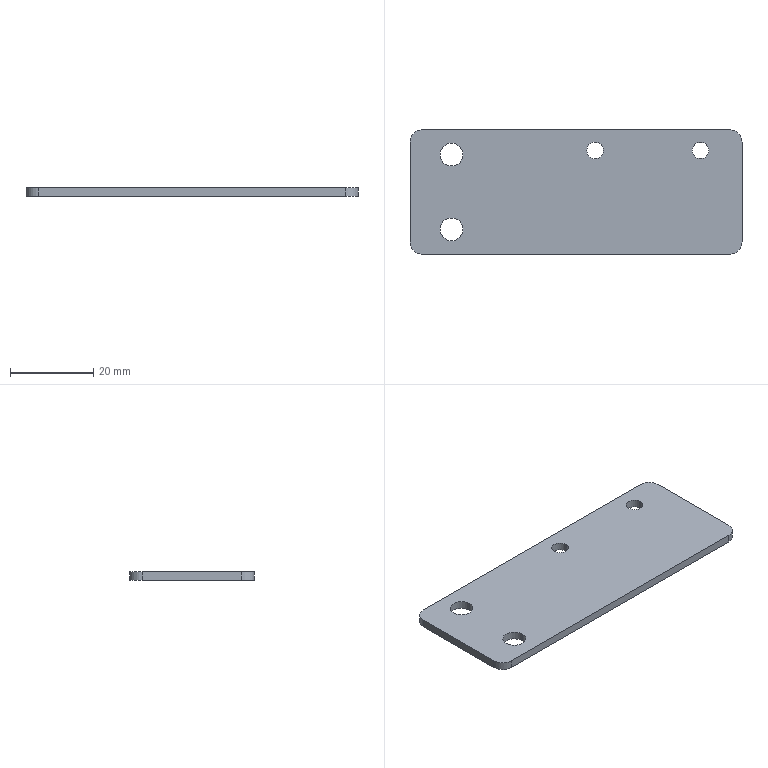Part | SolidWorks | features HoleWzd 2, Fillet 1, FlatPattern 1, SMBaseFlange 1, SheetMetal 1 | 1 solid | 18 faces | box 80 x 30 x 2 mm | volume 4639 mm3 | cylinder 12 | plane 6 | commonest cylinder face diameters 4 x4 5.5 x4 6 x4
STEP:
#1=CARTESIAN_POINT('',(7.25,24.,-2.));
#2=VERTEX_POINT('',#1);
#3=CARTESIAN_POINT('',(12.75,24.,-2.));
#4=VERTEX_POINT('',#3);
#5=CARTESIAN_POINT('',(10.,24.,-2.));
#6=DIRECTION('',(0.,0.,1.));
#7=DIRECTION('',(1.,0.,0.));
#8=AXIS2_PLACEMENT_3D('',#5,#6,#7);
#9=CIRCLE('',#8,2.75);
#10=EDGE_CURVE('',#2,#4,#9,.T.);
#11=ORIENTED_EDGE('',*,*,#10,.F.);
#12=CARTESIAN_POINT('',(7.25,24.,0.));
#13=VERTEX_POINT('',#12);
#14=CARTESIAN_POINT('',(7.25,24.,0.));
#15=DIRECTION('',(0.,0.,1.));
#16=VECTOR('',#15,1000.);
#17=LINE('',#14,#16);
#18=EDGE_CURVE('',#2,#13,#17,.T.);
#19=ORIENTED_EDGE('',*,*,#18,.T.);
#20=CARTESIAN_POINT('',(12.75,24.,0.));
#21=VERTEX_POINT('',#20);
#22=CARTESIAN_POINT('',(10.,24.,0.));
#23=DIRECTION('',(0.,0.,1.));
#24=DIRECTION('',(1.,0.,0.));
#25=AXIS2_PLACEMENT_3D('',#22,#23,#24);
#26=CIRCLE('',#25,2.75);
#27=EDGE_CURVE('',#13,#21,#26,.T.);
#28=ORIENTED_EDGE('',*,*,#27,.T.);
#29=CARTESIAN_POINT('',(12.75,24.,0.));
#30=DIRECTION('',(0.,0.,1.));
#31=VECTOR('',#30,1000.);
#32=LINE('',#29,#31);
#33=EDGE_CURVE('',#4,#21,#32,.T.);
#34=ORIENTED_EDGE('',*,*,#33,.F.);
#35=EDGE_LOOP('',(#11,#19,#28,#34));
#36=FACE_OUTER_BOUND('',#35,.T.);
#37=CARTESIAN_POINT('',(10.,24.,0.));
#38=DIRECTION('',(0.,0.,1.));
#39=DIRECTION('',(1.,0.,0.));
#40=AXIS2_PLACEMENT_3D('',#37,#38,#39);
#41=CYLINDRICAL_SURFACE('',#40,2.75);
#42=ADVANCED_FACE('',(#36),#41,.F.);
#43=CARTESIAN_POINT('',(7.25,6.,-2.));
#44=VERTEX_POINT('',#43);
#45=CARTESIAN_POINT('',(12.75,6.,-2.));
#46=VERTEX_POINT('',#45);
#47=CARTESIAN_POINT('',(10.,6.,-2.));
#48=DIRECTION('',(0.,0.,1.));
#49=DIRECTION('',(1.,0.,0.));
#50=AXIS2_PLACEMENT_3D('',#47,#48,#49);
#51=CIRCLE('',#50,2.75);
#52=EDGE_CURVE('',#44,#46,#51,.T.);
#53=ORIENTED_EDGE('',*,*,#52,.F.);
#54=CARTESIAN_POINT('',(7.25,6.,0.));
#55=VERTEX_POINT('',#54);
#56=CARTESIAN_POINT('',(7.25,6.,0.));
#57=DIRECTION('',(0.,0.,1.));
#58=VECTOR('',#57,1000.);
#59=LINE('',#56,#58);
#60=EDGE_CURVE('',#44,#55,#59,.T.);
#61=ORIENTED_EDGE('',*,*,#60,.T.);
#62=CARTESIAN_POINT('',(12.75,6.,0.));
#63=VERTEX_POINT('',#62);
#64=CARTESIAN_POINT('',(10.,6.,0.));
#65=DIRECTION('',(0.,0.,1.));
#66=DIRECTION('',(1.,0.,0.));
#67=AXIS2_PLACEMENT_3D('',#64,#65,#66);
#68=CIRCLE('',#67,2.75);
#69=EDGE_CURVE('',#55,#63,#68,.T.);
#70=ORIENTED_EDGE('',*,*,#69,.T.);
#71=CARTESIAN_POINT('',(12.75,6.,0.));
#72=DIRECTION('',(0.,0.,1.));
#73=VECTOR('',#72,1000.);
#74=LINE('',#71,#73);
#75=EDGE_CURVE('',#46,#63,#74,.T.);
#76=ORIENTED_EDGE('',*,*,#75,.F.);
#77=EDGE_LOOP('',(#53,#61,#70,#76));
#78=FACE_OUTER_BOUND('',#77,.T.);
#79=CARTESIAN_POINT('',(10.,6.,0.));
#80=DIRECTION('',(0.,0.,1.));
#81=DIRECTION('',(1.,0.,0.));
#82=AXIS2_PLACEMENT_3D('',#79,#80,#81);
#83=CYLINDRICAL_SURFACE('',#82,2.75);
#84=ADVANCED_FACE('',(#78),#83,.F.);
#85=CARTESIAN_POINT('',(72.,25.,-2.));
#86=VERTEX_POINT('',#85);
#87=CARTESIAN_POINT('',(68.,25.,-2.));
#88=VERTEX_POINT('',#87);
#89=CARTESIAN_POINT('',(70.,25.,-2.));
#90=DIRECTION('',(0.,0.,-1.));
#91=DIRECTION('',(-1.,0.,0.));
#92=AXIS2_PLACEMENT_3D('',#89,#90,#91);
#93=CIRCLE('',#92,2.);
#94=EDGE_CURVE('',#86,#88,#93,.T.);
#95=ORIENTED_EDGE('',*,*,#94,.T.);
#96=CARTESIAN_POINT('',(68.,25.,0.));
#97=VERTEX_POINT('',#96);
#98=CARTESIAN_POINT('',(68.,25.,0.));
#99=DIRECTION('',(0.,0.,1.));
#100=VECTOR('',#99,1000.);
#101=LINE('',#98,#100);
#102=EDGE_CURVE('',#88,#97,#101,.T.);
#103=ORIENTED_EDGE('',*,*,#102,.T.);
#104=CARTESIAN_POINT('',(72.,25.,0.));
#105=VERTEX_POINT('',#104);
#106=CARTESIAN_POINT('',(70.,25.,0.));
#107=DIRECTION('',(0.,0.,1.));
#108=DIRECTION('',(1.,0.,0.));
#109=AXIS2_PLACEMENT_3D('',#106,#107,#108);
#110=CIRCLE('',#109,2.);
#111=EDGE_CURVE('',#97,#105,#110,.T.);
#112=ORIENTED_EDGE('',*,*,#111,.T.);
#113=CARTESIAN_POINT('',(72.,25.,0.));
#114=DIRECTION('',(0.,0.,1.));
#115=VECTOR('',#114,1000.);
#116=LINE('',#113,#115);
#117=EDGE_CURVE('',#86,#105,#116,.T.);
#118=ORIENTED_EDGE('',*,*,#117,.F.);
#119=EDGE_LOOP('',(#95,#103,#112,#118));
#120=FACE_OUTER_BOUND('',#119,.T.);
#121=CARTESIAN_POINT('',(70.,25.,0.));
#122=DIRECTION('',(0.,0.,1.));
#123=DIRECTION('',(1.,0.,0.));
#124=AXIS2_PLACEMENT_3D('',#121,#122,#123);
#125=CYLINDRICAL_SURFACE('',#124,2.);
#126=ADVANCED_FACE('',(#120),#125,.F.);
#127=CARTESIAN_POINT('',(46.6,25.,-2.));
#128=VERTEX_POINT('',#127);
#129=CARTESIAN_POINT('',(42.6,25.,-2.));
#130=VERTEX_POINT('',#129);
#131=CARTESIAN_POINT('',(44.6,25.,-2.));
#132=DIRECTION('',(0.,0.,-1.));
#133=DIRECTION('',(-1.,0.,0.));
#134=AXIS2_PLACEMENT_3D('',#131,#132,#133);
#135=CIRCLE('',#134,2.);
#136=EDGE_CURVE('',#128,#130,#135,.T.);
#137=ORIENTED_EDGE('',*,*,#136,.T.);
#138=CARTESIAN_POINT('',(42.6,25.,0.));
#139=VERTEX_POINT('',#138);
#140=CARTESIAN_POINT('',(42.6,25.,0.));
#141=DIRECTION('',(0.,0.,1.));
#142=VECTOR('',#141,1000.);
#143=LINE('',#140,#142);
#144=EDGE_CURVE('',#130,#139,#143,.T.);
#145=ORIENTED_EDGE('',*,*,#144,.T.);
#146=CARTESIAN_POINT('',(46.6,25.,0.));
#147=VERTEX_POINT('',#146);
#148=CARTESIAN_POINT('',(44.6,25.,0.));
#149=DIRECTION('',(0.,0.,1.));
#150=DIRECTION('',(1.,0.,0.));
#151=AXIS2_PLACEMENT_3D('',#148,#149,#150);
#152=CIRCLE('',#151,2.);
#153=EDGE_CURVE('',#139,#147,#152,.T.);
#154=ORIENTED_EDGE('',*,*,#153,.T.);
#155=CARTESIAN_POINT('',(46.6,25.,0.));
#156=DIRECTION('',(0.,0.,1.));
#157=VECTOR('',#156,1000.);
#158=LINE('',#155,#157);
#159=EDGE_CURVE('',#128,#147,#158,.T.);
#160=ORIENTED_EDGE('',*,*,#159,.F.);
#161=EDGE_LOOP('',(#137,#145,#154,#160));
#162=FACE_OUTER_BOUND('',#161,.T.);
#163=CARTESIAN_POINT('',(44.6,25.,0.));
#164=DIRECTION('',(0.,0.,1.));
#165=DIRECTION('',(1.,0.,0.));
#166=AXIS2_PLACEMENT_3D('',#163,#164,#165);
#167=CYLINDRICAL_SURFACE('',#166,2.);
#168=ADVANCED_FACE('',(#162),#167,.F.);
#169=CARTESIAN_POINT('',(0.,27.,-2.));
#170=VERTEX_POINT('',#169);
#171=CARTESIAN_POINT('',(0.,3.,-2.));
#172=VERTEX_POINT('',#171);
#173=CARTESIAN_POINT('',(0.,0.,-2.));
#174=DIRECTION('',(0.,-1.,0.));
#175=VECTOR('',#174,1000.);
#176=LINE('',#173,#175);
#177=EDGE_CURVE('',#170,#172,#176,.T.);
#178=ORIENTED_EDGE('',*,*,#177,.T.);
#179=CARTESIAN_POINT('',(0.,3.,0.));
#180=VERTEX_POINT('',#179);
#181=CARTESIAN_POINT('',(0.,3.,-2.));
#182=DIRECTION('',(0.,0.,1.));
#183=VECTOR('',#182,1000.);
#184=LINE('',#181,#183);
#185=EDGE_CURVE('',#172,#180,#184,.T.);
#186=ORIENTED_EDGE('',*,*,#185,.T.);
#187=CARTESIAN_POINT('',(0.,27.,0.));
#188=VERTEX_POINT('',#187);
#189=CARTESIAN_POINT('',(0.,0.,0.));
#190=DIRECTION('',(0.,-1.,0.));
#191=VECTOR('',#190,1000.);
#192=LINE('',#189,#191);
#193=EDGE_CURVE('',#188,#180,#192,.T.);
#194=ORIENTED_EDGE('',*,*,#193,.F.);
#195=CARTESIAN_POINT('',(0.,27.,-2.));
#196=DIRECTION('',(0.,0.,-1.));
#197=VECTOR('',#196,1000.);
#198=LINE('',#195,#197);
#199=EDGE_CURVE('',#188,#170,#198,.T.);
#200=ORIENTED_EDGE('',*,*,#199,.T.);
#201=EDGE_LOOP('',(#178,#186,#194,#200));
#202=FACE_OUTER_BOUND('',#201,.T.);
#203=CARTESIAN_POINT('',(0.,0.,-2.));
#204=DIRECTION('',(-1.,0.,0.));
#205=DIRECTION('',(0.,0.,1.));
#206=AXIS2_PLACEMENT_3D('',#203,#204,#205);
#207=PLANE('',#206);
#208=ADVANCED_FACE('',(#202),#207,.T.);
#209=CARTESIAN_POINT('',(77.,30.,0.));
#210=VERTEX_POINT('',#209);
#211=CARTESIAN_POINT('',(3.,30.,0.));
#212=VERTEX_POINT('',#211);
#213=CARTESIAN_POINT('',(0.,30.,0.));
#214=DIRECTION('',(-1.,0.,0.));
#215=VECTOR('',#214,1000.);
#216=LINE('',#213,#215);
#217=EDGE_CURVE('',#210,#212,#216,.T.);
#218=ORIENTED_EDGE('',*,*,#217,.F.);
#219=CARTESIAN_POINT('',(77.,30.,-2.));
#220=VERTEX_POINT('',#219);
#221=CARTESIAN_POINT('',(77.,30.,-2.));
#222=DIRECTION('',(0.,0.,-1.));
#223=VECTOR('',#222,1000.);
#224=LINE('',#221,#223);
#225=EDGE_CURVE('',#210,#220,#224,.T.);
#226=ORIENTED_EDGE('',*,*,#225,.T.);
#227=CARTESIAN_POINT('',(3.,30.,-2.));
#228=VERTEX_POINT('',#227);
#229=CARTESIAN_POINT('',(0.,30.,-2.));
#230=DIRECTION('',(-1.,0.,0.));
#231=VECTOR('',#230,1000.);
#232=LINE('',#229,#231);
#233=EDGE_CURVE('',#220,#228,#232,.T.);
#234=ORIENTED_EDGE('',*,*,#233,.T.);
#235=CARTESIAN_POINT('',(3.,30.,-2.));
#236=DIRECTION('',(0.,0.,1.));
#237=VECTOR('',#236,1000.);
#238=LINE('',#235,#237);
#239=EDGE_CURVE('',#228,#212,#238,.T.);
#240=ORIENTED_EDGE('',*,*,#239,.T.);
#241=EDGE_LOOP('',(#218,#226,#234,#240));
#242=FACE_OUTER_BOUND('',#241,.T.);
#243=CARTESIAN_POINT('',(0.,30.,-2.));
#244=DIRECTION('',(0.,1.,0.));
#245=DIRECTION('',(0.,0.,1.));
#246=AXIS2_PLACEMENT_3D('',#243,#244,#245);
#247=PLANE('',#246);
#248=ADVANCED_FACE('',(#242),#247,.T.);
#249=CARTESIAN_POINT('',(80.,3.,0.));
#250=VERTEX_POINT('',#249);
#251=CARTESIAN_POINT('',(80.,27.,0.));
#252=VERTEX_POINT('',#251);
#253=CARTESIAN_POINT('',(80.,0.,0.));
#254=DIRECTION('',(0.,1.,0.));
#255=VECTOR('',#254,1000.);
#256=LINE('',#253,#255);
#257=EDGE_CURVE('',#250,#252,#256,.T.);
#258=ORIENTED_EDGE('',*,*,#257,.F.);
#259=CARTESIAN_POINT('',(80.,3.,-2.));
#260=VERTEX_POINT('',#259);
#261=CARTESIAN_POINT('',(80.,3.,-2.));
#262=DIRECTION('',(0.,0.,-1.));
#263=VECTOR('',#262,1000.);
#264=LINE('',#261,#263);
#265=EDGE_CURVE('',#250,#260,#264,.T.);
#266=ORIENTED_EDGE('',*,*,#265,.T.);
#267=CARTESIAN_POINT('',(80.,27.,-2.));
#268=VERTEX_POINT('',#267);
#269=CARTESIAN_POINT('',(80.,0.,-2.));
#270=DIRECTION('',(0.,1.,0.));
#271=VECTOR('',#270,1000.);
#272=LINE('',#269,#271);
#273=EDGE_CURVE('',#260,#268,#272,.T.);
#274=ORIENTED_EDGE('',*,*,#273,.T.);
#275=CARTESIAN_POINT('',(80.,27.,-2.));
#276=DIRECTION('',(0.,0.,1.));
#277=VECTOR('',#276,1000.);
#278=LINE('',#275,#277);
#279=EDGE_CURVE('',#268,#252,#278,.T.);
#280=ORIENTED_EDGE('',*,*,#279,.T.);
#281=EDGE_LOOP('',(#258,#266,#274,#280));
#282=FACE_OUTER_BOUND('',#281,.T.);
#283=CARTESIAN_POINT('',(80.,0.,-2.));
#284=DIRECTION('',(1.,0.,0.));
#285=DIRECTION('',(0.,0.,-1.));
#286=AXIS2_PLACEMENT_3D('',#283,#284,#285);
#287=PLANE('',#286);
#288=ADVANCED_FACE('',(#282),#287,.T.);
#289=CARTESIAN_POINT('',(3.,0.,-2.));
#290=VERTEX_POINT('',#289);
#291=CARTESIAN_POINT('',(77.,0.,-2.));
#292=VERTEX_POINT('',#291);
#293=CARTESIAN_POINT('',(0.,0.,-2.));
#294=DIRECTION('',(1.,0.,0.));
#295=VECTOR('',#294,1000.);
#296=LINE('',#293,#295);
#297=EDGE_CURVE('',#290,#292,#296,.T.);
#298=ORIENTED_EDGE('',*,*,#297,.T.);
#299=CARTESIAN_POINT('',(77.,0.,0.));
#300=VERTEX_POINT('',#299);
#301=CARTESIAN_POINT('',(77.,0.,-2.));
#302=DIRECTION('',(0.,0.,1.));
#303=VECTOR('',#302,1000.);
#304=LINE('',#301,#303);
#305=EDGE_CURVE('',#292,#300,#304,.T.);
#306=ORIENTED_EDGE('',*,*,#305,.T.);
#307=CARTESIAN_POINT('',(3.,0.,0.));
#308=VERTEX_POINT('',#307);
#309=CARTESIAN_POINT('',(0.,0.,0.));
#310=DIRECTION('',(1.,0.,0.));
#311=VECTOR('',#310,1000.);
#312=LINE('',#309,#311);
#313=EDGE_CURVE('',#308,#300,#312,.T.);
#314=ORIENTED_EDGE('',*,*,#313,.F.);
#315=CARTESIAN_POINT('',(3.,0.,-2.));
#316=DIRECTION('',(0.,0.,-1.));
#317=VECTOR('',#316,1000.);
#318=LINE('',#315,#317);
#319=EDGE_CURVE('',#308,#290,#318,.T.);
#320=ORIENTED_EDGE('',*,*,#319,.T.);
#321=EDGE_LOOP('',(#298,#306,#314,#320));
#322=FACE_OUTER_BOUND('',#321,.T.);
#323=CARTESIAN_POINT('',(0.,0.,-2.));
#324=DIRECTION('',(0.,-1.,0.));
#325=DIRECTION('',(0.,0.,-1.));
#326=AXIS2_PLACEMENT_3D('',#323,#324,#325);
#327=PLANE('',#326);
#328=ADVANCED_FACE('',(#322),#327,.T.);
#329=CARTESIAN_POINT('',(10.,24.,-2.));
#330=DIRECTION('',(0.,0.,1.));
#331=DIRECTION('',(1.,0.,0.));
#332=AXIS2_PLACEMENT_3D('',#329,#330,#331);
#333=CIRCLE('',#332,2.75);
#334=EDGE_CURVE('',#4,#2,#333,.T.);
#335=ORIENTED_EDGE('',*,*,#334,.T.);
#336=ORIENTED_EDGE('',*,*,#10,.T.);
#337=EDGE_LOOP('',(#335,#336));
#338=FACE_BOUND('',#337,.T.);
#339=CARTESIAN_POINT('',(10.,6.,-2.));
#340=DIRECTION('',(0.,0.,1.));
#341=DIRECTION('',(1.,0.,0.));
#342=AXIS2_PLACEMENT_3D('',#339,#340,#341);
#343=CIRCLE('',#342,2.75);
#344=EDGE_CURVE('',#46,#44,#343,.T.);
#345=ORIENTED_EDGE('',*,*,#344,.T.);
#346=ORIENTED_EDGE('',*,*,#52,.T.);
#347=EDGE_LOOP('',(#345,#346));
#348=FACE_BOUND('',#347,.T.);
#349=ORIENTED_EDGE('',*,*,#94,.F.);
#350=CARTESIAN_POINT('',(70.,25.,-2.));
#351=DIRECTION('',(0.,0.,-1.));
#352=DIRECTION('',(-1.,0.,0.));
#353=AXIS2_PLACEMENT_3D('',#350,#351,#352);
#354=CIRCLE('',#353,2.);
#355=EDGE_CURVE('',#88,#86,#354,.T.);
#356=ORIENTED_EDGE('',*,*,#355,.F.);
#357=EDGE_LOOP('',(#349,#356));
#358=FACE_BOUND('',#357,.T.);
#359=ORIENTED_EDGE('',*,*,#136,.F.);
#360=CARTESIAN_POINT('',(44.6,25.,-2.));
#361=DIRECTION('',(0.,0.,-1.));
#362=DIRECTION('',(-1.,0.,0.));
#363=AXIS2_PLACEMENT_3D('',#360,#361,#362);
#364=CIRCLE('',#363,2.);
#365=EDGE_CURVE('',#130,#128,#364,.T.);
#366=ORIENTED_EDGE('',*,*,#365,.F.);
#367=EDGE_LOOP('',(#359,#366));
#368=FACE_BOUND('',#367,.T.);
#369=ORIENTED_EDGE('',*,*,#273,.F.);
#370=CARTESIAN_POINT('',(77.,3.,-2.));
#371=DIRECTION('',(0.,0.,-1.));
#372=DIRECTION('',(-1.,0.,0.));
#373=AXIS2_PLACEMENT_3D('',#370,#371,#372);
#374=CIRCLE('',#373,3.);
#375=EDGE_CURVE('',#260,#292,#374,.T.);
#376=ORIENTED_EDGE('',*,*,#375,.T.);
#377=ORIENTED_EDGE('',*,*,#297,.F.);
#378=CARTESIAN_POINT('',(3.,3.,-2.));
#379=DIRECTION('',(0.,0.,-1.));
#380=DIRECTION('',(-1.,0.,0.));
#381=AXIS2_PLACEMENT_3D('',#378,#379,#380);
#382=CIRCLE('',#381,3.);
#383=EDGE_CURVE('',#290,#172,#382,.T.);
#384=ORIENTED_EDGE('',*,*,#383,.T.);
#385=ORIENTED_EDGE('',*,*,#177,.F.);
#386=CARTESIAN_POINT('',(3.,27.,-2.));
#387=DIRECTION('',(0.,0.,-1.));
#388=DIRECTION('',(-1.,0.,0.));
#389=AXIS2_PLACEMENT_3D('',#386,#387,#388);
#390=CIRCLE('',#389,3.);
#391=EDGE_CURVE('',#170,#228,#390,.T.);
#392=ORIENTED_EDGE('',*,*,#391,.T.);
#393=ORIENTED_EDGE('',*,*,#233,.F.);
#394=CARTESIAN_POINT('',(77.,27.,-2.));
#395=DIRECTION('',(0.,0.,-1.));
#396=DIRECTION('',(-1.,0.,0.));
#397=AXIS2_PLACEMENT_3D('',#394,#395,#396);
#398=CIRCLE('',#397,3.);
#399=EDGE_CURVE('',#220,#268,#398,.T.);
#400=ORIENTED_EDGE('',*,*,#399,.T.);
#401=EDGE_LOOP('',(#369,#376,#377,#384,#385,#392,#393,#400));
#402=FACE_OUTER_BOUND('',#401,.T.);
#403=CARTESIAN_POINT('',(0.,0.,-2.));
#404=DIRECTION('',(0.,0.,-1.));
#405=DIRECTION('',(-1.,0.,0.));
#406=AXIS2_PLACEMENT_3D('',#403,#404,#405);
#407=PLANE('',#406);
#408=ADVANCED_FACE('',(#338,#348,#358,#368,#402),#407,.T.);
#409=CARTESIAN_POINT('',(10.,24.,0.));
#410=DIRECTION('',(0.,0.,1.));
#411=DIRECTION('',(1.,0.,0.));
#412=AXIS2_PLACEMENT_3D('',#409,#410,#411);
#413=CIRCLE('',#412,2.75);
#414=EDGE_CURVE('',#21,#13,#413,.T.);
#415=ORIENTED_EDGE('',*,*,#414,.F.);
#416=ORIENTED_EDGE('',*,*,#27,.F.);
#417=EDGE_LOOP('',(#415,#416));
#418=FACE_BOUND('',#417,.T.);
#419=CARTESIAN_POINT('',(10.,6.,0.));
#420=DIRECTION('',(0.,0.,1.));
#421=DIRECTION('',(1.,0.,0.));
#422=AXIS2_PLACEMENT_3D('',#419,#420,#421);
#423=CIRCLE('',#422,2.75);
#424=EDGE_CURVE('',#63,#55,#423,.T.);
#425=ORIENTED_EDGE('',*,*,#424,.F.);
#426=ORIENTED_EDGE('',*,*,#69,.F.);
#427=EDGE_LOOP('',(#425,#426));
#428=FACE_BOUND('',#427,.T.);
#429=CARTESIAN_POINT('',(70.,25.,0.));
#430=DIRECTION('',(0.,0.,1.));
#431=DIRECTION('',(1.,0.,0.));
#432=AXIS2_PLACEMENT_3D('',#429,#430,#431);
#433=CIRCLE('',#432,2.);
#434=EDGE_CURVE('',#105,#97,#433,.T.);
#435=ORIENTED_EDGE('',*,*,#434,.F.);
#436=ORIENTED_EDGE('',*,*,#111,.F.);
#437=EDGE_LOOP('',(#435,#436));
#438=FACE_BOUND('',#437,.T.);
#439=CARTESIAN_POINT('',(44.6,25.,0.));
#440=DIRECTION('',(0.,0.,1.));
#441=DIRECTION('',(1.,0.,0.));
#442=AXIS2_PLACEMENT_3D('',#439,#440,#441);
#443=CIRCLE('',#442,2.);
#444=EDGE_CURVE('',#147,#139,#443,.T.);
#445=ORIENTED_EDGE('',*,*,#444,.F.);
#446=ORIENTED_EDGE('',*,*,#153,.F.);
#447=EDGE_LOOP('',(#445,#446));
#448=FACE_BOUND('',#447,.T.);
#449=ORIENTED_EDGE('',*,*,#313,.T.);
#450=CARTESIAN_POINT('',(77.,3.,0.));
#451=DIRECTION('',(0.,0.,1.));
#452=DIRECTION('',(-1.,0.,0.));
#453=AXIS2_PLACEMENT_3D('',#450,#451,#452);
#454=CIRCLE('',#453,3.);
#455=EDGE_CURVE('',#300,#250,#454,.T.);
#456=ORIENTED_EDGE('',*,*,#455,.T.);
#457=ORIENTED_EDGE('',*,*,#257,.T.);
#458=CARTESIAN_POINT('',(77.,27.,0.));
#459=DIRECTION('',(0.,0.,1.));
#460=DIRECTION('',(-1.,0.,0.));
#461=AXIS2_PLACEMENT_3D('',#458,#459,#460);
#462=CIRCLE('',#461,3.);
#463=EDGE_CURVE('',#252,#210,#462,.T.);
#464=ORIENTED_EDGE('',*,*,#463,.T.);
#465=ORIENTED_EDGE('',*,*,#217,.T.);
#466=CARTESIAN_POINT('',(3.,27.,0.));
#467=DIRECTION('',(0.,0.,1.));
#468=DIRECTION('',(-1.,0.,0.));
#469=AXIS2_PLACEMENT_3D('',#466,#467,#468);
#470=CIRCLE('',#469,3.);
#471=EDGE_CURVE('',#212,#188,#470,.T.);
#472=ORIENTED_EDGE('',*,*,#471,.T.);
#473=ORIENTED_EDGE('',*,*,#193,.T.);
#474=CARTESIAN_POINT('',(3.,3.,0.));
#475=DIRECTION('',(0.,0.,1.));
#476=DIRECTION('',(-1.,0.,0.));
#477=AXIS2_PLACEMENT_3D('',#474,#475,#476);
#478=CIRCLE('',#477,3.);
#479=EDGE_CURVE('',#180,#308,#478,.T.);
#480=ORIENTED_EDGE('',*,*,#479,.T.);
#481=EDGE_LOOP('',(#449,#456,#457,#464,#465,#472,#473,#480));
#482=FACE_OUTER_BOUND('',#481,.T.);
#483=CARTESIAN_POINT('',(0.,0.,0.));
#484=DIRECTION('',(0.,0.,-1.));
#485=DIRECTION('',(-1.,0.,0.));
#486=AXIS2_PLACEMENT_3D('',#483,#484,#485);
#487=PLANE('',#486);
#488=ADVANCED_FACE('',(#418,#428,#438,#448,#482),#487,.F.);
#489=ORIENTED_EDGE('',*,*,#144,.F.);
#490=ORIENTED_EDGE('',*,*,#365,.T.);
#491=ORIENTED_EDGE('',*,*,#159,.T.);
#492=ORIENTED_EDGE('',*,*,#444,.T.);
#493=EDGE_LOOP('',(#489,#490,#491,#492));
#494=FACE_OUTER_BOUND('',#493,.T.);
#495=CARTESIAN_POINT('',(44.6,25.,0.));
#496=DIRECTION('',(0.,0.,1.));
#497=DIRECTION('',(1.,0.,0.));
#498=AXIS2_PLACEMENT_3D('',#495,#496,#497);
#499=CYLINDRICAL_SURFACE('',#498,2.);
#500=ADVANCED_FACE('',(#494),#499,.F.);
#501=ORIENTED_EDGE('',*,*,#102,.F.);
#502=ORIENTED_EDGE('',*,*,#355,.T.);
#503=ORIENTED_EDGE('',*,*,#117,.T.);
#504=ORIENTED_EDGE('',*,*,#434,.T.);
#505=EDGE_LOOP('',(#501,#502,#503,#504));
#506=FACE_OUTER_BOUND('',#505,.T.);
#507=CARTESIAN_POINT('',(70.,25.,0.));
#508=DIRECTION('',(0.,0.,1.));
#509=DIRECTION('',(1.,0.,0.));
#510=AXIS2_PLACEMENT_3D('',#507,#508,#509);
#511=CYLINDRICAL_SURFACE('',#510,2.);
#512=ADVANCED_FACE('',(#506),#511,.F.);
#513=ORIENTED_EDGE('',*,*,#60,.F.);
#514=ORIENTED_EDGE('',*,*,#344,.F.);
#515=ORIENTED_EDGE('',*,*,#75,.T.);
#516=ORIENTED_EDGE('',*,*,#424,.T.);
#517=EDGE_LOOP('',(#513,#514,#515,#516));
#518=FACE_OUTER_BOUND('',#517,.T.);
#519=CARTESIAN_POINT('',(10.,6.,0.));
#520=DIRECTION('',(0.,0.,1.));
#521=DIRECTION('',(1.,0.,0.));
#522=AXIS2_PLACEMENT_3D('',#519,#520,#521);
#523=CYLINDRICAL_SURFACE('',#522,2.75);
#524=ADVANCED_FACE('',(#518),#523,.F.);
#525=ORIENTED_EDGE('',*,*,#18,.F.);
#526=ORIENTED_EDGE('',*,*,#334,.F.);
#527=ORIENTED_EDGE('',*,*,#33,.T.);
#528=ORIENTED_EDGE('',*,*,#414,.T.);
#529=EDGE_LOOP('',(#525,#526,#527,#528));
#530=FACE_OUTER_BOUND('',#529,.T.);
#531=CARTESIAN_POINT('',(10.,24.,0.));
#532=DIRECTION('',(0.,0.,1.));
#533=DIRECTION('',(1.,0.,0.));
#534=AXIS2_PLACEMENT_3D('',#531,#532,#533);
#535=CYLINDRICAL_SURFACE('',#534,2.75);
#536=ADVANCED_FACE('',(#530),#535,.F.);
#537=ORIENTED_EDGE('',*,*,#375,.F.);
#538=ORIENTED_EDGE('',*,*,#265,.F.);
#539=ORIENTED_EDGE('',*,*,#455,.F.);
#540=ORIENTED_EDGE('',*,*,#305,.F.);
#541=EDGE_LOOP('',(#537,#538,#539,#540));
#542=FACE_OUTER_BOUND('',#541,.T.);
#543=CARTESIAN_POINT('',(77.,3.,-2.));
#544=DIRECTION('',(0.,0.,1.));
#545=DIRECTION('',(1.,0.,0.));
#546=AXIS2_PLACEMENT_3D('',#543,#544,#545);
#547=CYLINDRICAL_SURFACE('',#546,3.);
#548=ADVANCED_FACE('',(#542),#547,.T.);
#549=ORIENTED_EDGE('',*,*,#399,.F.);
#550=ORIENTED_EDGE('',*,*,#225,.F.);
#551=ORIENTED_EDGE('',*,*,#463,.F.);
#552=ORIENTED_EDGE('',*,*,#279,.F.);
#553=EDGE_LOOP('',(#549,#550,#551,#552));
#554=FACE_OUTER_BOUND('',#553,.T.);
#555=CARTESIAN_POINT('',(77.,27.,-2.));
#556=DIRECTION('',(0.,0.,1.));
#557=DIRECTION('',(1.,0.,0.));
#558=AXIS2_PLACEMENT_3D('',#555,#556,#557);
#559=CYLINDRICAL_SURFACE('',#558,3.);
#560=ADVANCED_FACE('',(#554),#559,.T.);
#561=ORIENTED_EDGE('',*,*,#383,.F.);
#562=ORIENTED_EDGE('',*,*,#319,.F.);
#563=ORIENTED_EDGE('',*,*,#479,.F.);
#564=ORIENTED_EDGE('',*,*,#185,.F.);
#565=EDGE_LOOP('',(#561,#562,#563,#564));
#566=FACE_OUTER_BOUND('',#565,.T.);
#567=CARTESIAN_POINT('',(3.,3.,-2.));
#568=DIRECTION('',(0.,0.,1.));
#569=DIRECTION('',(1.,0.,0.));
#570=AXIS2_PLACEMENT_3D('',#567,#568,#569);
#571=CYLINDRICAL_SURFACE('',#570,3.);
#572=ADVANCED_FACE('',(#566),#571,.T.);
#573=ORIENTED_EDGE('',*,*,#391,.F.);
#574=ORIENTED_EDGE('',*,*,#199,.F.);
#575=ORIENTED_EDGE('',*,*,#471,.F.);
#576=ORIENTED_EDGE('',*,*,#239,.F.);
#577=EDGE_LOOP('',(#573,#574,#575,#576));
#578=FACE_OUTER_BOUND('',#577,.T.);
#579=CARTESIAN_POINT('',(3.,27.,-2.));
#580=DIRECTION('',(0.,0.,1.));
#581=DIRECTION('',(1.,0.,0.));
#582=AXIS2_PLACEMENT_3D('',#579,#580,#581);
#583=CYLINDRICAL_SURFACE('',#582,3.);
#584=ADVANCED_FACE('',(#578),#583,.T.);
#585=CLOSED_SHELL('',(#42,#84,#126,#168,#208,#248,#288,#328,#408,#488,#500,#512,#524,#536,#548,#560,#572,#584));
#586=MANIFOLD_SOLID_BREP('',#585);
#587=CARTESIAN_POINT('',(0.,0.,0.));
#588=DIRECTION('',(0.,0.,1.));
#589=DIRECTION('',(1.,0.,0.));
#590=AXIS2_PLACEMENT_3D('',#587,#588,#589);
#591=(LENGTH_UNIT()NAMED_UNIT(*)SI_UNIT(.MILLI.,.METRE.));
#592=UNCERTAINTY_MEASURE_WITH_UNIT(LENGTH_MEASURE(0.00001),#591,'','');
#593=(NAMED_UNIT(*)PLANE_ANGLE_UNIT()SI_UNIT($,.RADIAN.));
#594=(NAMED_UNIT(*)SI_UNIT($,.STERADIAN.)SOLID_ANGLE_UNIT());
#595=(GEOMETRIC_REPRESENTATION_CONTEXT(3)GLOBAL_UNCERTAINTY_ASSIGNED_CONTEXT((#592))GLOBAL_UNIT_ASSIGNED_CONTEXT((#591,#593,#594))REPRESENTATION_CONTEXT('',''));
#596=ADVANCED_BREP_SHAPE_REPRESENTATION('',(#586,#590),#595);